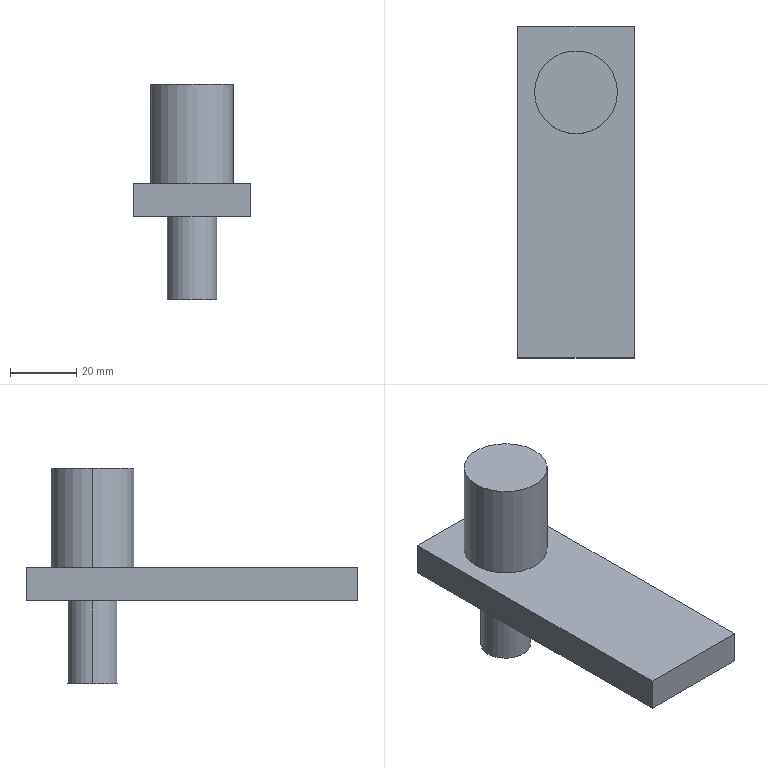Part | SolidWorks | features ICE 2, Extrusion 1 | 1 solid | 12 faces | box 35 x 100 x 65 mm | volume 54144 mm3 | plane 8 | cylinder 4 | commonest cylinder face diameters 15 x2 25 x2
STEP:
#1=CARTESIAN_POINT('',(-7.5,30.,-25.));
#2=VERTEX_POINT('',#1);
#3=CARTESIAN_POINT('',(7.5,30.,-25.));
#4=VERTEX_POINT('',#3);
#5=CARTESIAN_POINT('',(0.,30.,-25.));
#6=DIRECTION('',(0.,0.,-1.));
#7=DIRECTION('',(-1.,0.,0.));
#8=AXIS2_PLACEMENT_3D('',#5,#6,#7);
#9=CIRCLE('',#8,7.5);
#10=EDGE_CURVE('',#2,#4,#9,.T.);
#11=ORIENTED_EDGE('',*,*,#10,.F.);
#12=CARTESIAN_POINT('',(-7.5,30.,0.));
#13=VERTEX_POINT('',#12);
#14=CARTESIAN_POINT('',(-7.5,30.,-25.));
#15=DIRECTION('',(0.,0.,1.));
#16=VECTOR('',#15,1000.);
#17=LINE('',#14,#16);
#18=EDGE_CURVE('',#2,#13,#17,.T.);
#19=ORIENTED_EDGE('',*,*,#18,.T.);
#20=CARTESIAN_POINT('',(7.5,30.,0.));
#21=VERTEX_POINT('',#20);
#22=CARTESIAN_POINT('',(0.,30.,0.));
#23=DIRECTION('',(0.,0.,-1.));
#24=DIRECTION('',(-1.,0.,0.));
#25=AXIS2_PLACEMENT_3D('',#22,#23,#24);
#26=CIRCLE('',#25,7.5);
#27=EDGE_CURVE('',#13,#21,#26,.T.);
#28=ORIENTED_EDGE('',*,*,#27,.T.);
#29=CARTESIAN_POINT('',(7.5,30.,-25.));
#30=DIRECTION('',(0.,0.,1.));
#31=VECTOR('',#30,1000.);
#32=LINE('',#29,#31);
#33=EDGE_CURVE('',#4,#21,#32,.T.);
#34=ORIENTED_EDGE('',*,*,#33,.F.);
#35=EDGE_LOOP('',(#11,#19,#28,#34));
#36=FACE_OUTER_BOUND('',#35,.T.);
#37=CARTESIAN_POINT('',(0.,30.,-25.));
#38=DIRECTION('',(0.,0.,1.));
#39=DIRECTION('',(1.,0.,0.));
#40=AXIS2_PLACEMENT_3D('',#37,#38,#39);
#41=CYLINDRICAL_SURFACE('',#40,7.5);
#42=ADVANCED_FACE('',(#36),#41,.T.);
#43=CARTESIAN_POINT('',(12.5,30.,40.));
#44=VERTEX_POINT('',#43);
#45=CARTESIAN_POINT('',(-12.5,30.,40.));
#46=VERTEX_POINT('',#45);
#47=CARTESIAN_POINT('',(0.,30.,40.));
#48=DIRECTION('',(0.,0.,1.));
#49=DIRECTION('',(1.,0.,0.));
#50=AXIS2_PLACEMENT_3D('',#47,#48,#49);
#51=CIRCLE('',#50,12.5);
#52=EDGE_CURVE('',#44,#46,#51,.T.);
#53=ORIENTED_EDGE('',*,*,#52,.F.);
#54=CARTESIAN_POINT('',(12.5,30.,10.));
#55=VERTEX_POINT('',#54);
#56=CARTESIAN_POINT('',(12.5,30.,40.));
#57=DIRECTION('',(0.,0.,-1.));
#58=VECTOR('',#57,1000.);
#59=LINE('',#56,#58);
#60=EDGE_CURVE('',#44,#55,#59,.T.);
#61=ORIENTED_EDGE('',*,*,#60,.T.);
#62=CARTESIAN_POINT('',(-12.5,30.,10.));
#63=VERTEX_POINT('',#62);
#64=CARTESIAN_POINT('',(0.,30.,10.));
#65=DIRECTION('',(0.,0.,1.));
#66=DIRECTION('',(-1.,0.,0.));
#67=AXIS2_PLACEMENT_3D('',#64,#65,#66);
#68=CIRCLE('',#67,12.5);
#69=EDGE_CURVE('',#55,#63,#68,.T.);
#70=ORIENTED_EDGE('',*,*,#69,.T.);
#71=CARTESIAN_POINT('',(-12.5,30.,40.));
#72=DIRECTION('',(0.,0.,-1.));
#73=VECTOR('',#72,1000.);
#74=LINE('',#71,#73);
#75=EDGE_CURVE('',#46,#63,#74,.T.);
#76=ORIENTED_EDGE('',*,*,#75,.F.);
#77=EDGE_LOOP('',(#53,#61,#70,#76));
#78=FACE_OUTER_BOUND('',#77,.T.);
#79=CARTESIAN_POINT('',(0.,30.,40.));
#80=DIRECTION('',(0.,0.,-1.));
#81=DIRECTION('',(-1.,0.,0.));
#82=AXIS2_PLACEMENT_3D('',#79,#80,#81);
#83=CYLINDRICAL_SURFACE('',#82,12.5);
#84=ADVANCED_FACE('',(#78),#83,.T.);
#85=CARTESIAN_POINT('',(17.5,-50.,0.));
#86=VERTEX_POINT('',#85);
#87=CARTESIAN_POINT('',(17.5,50.,0.));
#88=VERTEX_POINT('',#87);
#89=CARTESIAN_POINT('',(17.5,-50.,0.));
#90=DIRECTION('',(0.,1.,0.));
#91=VECTOR('',#90,1000.);
#92=LINE('',#89,#91);
#93=EDGE_CURVE('',#86,#88,#92,.T.);
#94=ORIENTED_EDGE('',*,*,#93,.T.);
#95=CARTESIAN_POINT('',(17.5,50.,10.));
#96=VERTEX_POINT('',#95);
#97=CARTESIAN_POINT('',(17.5,50.,10.));
#98=DIRECTION('',(0.,0.,-1.));
#99=VECTOR('',#98,1000.);
#100=LINE('',#97,#99);
#101=EDGE_CURVE('',#96,#88,#100,.T.);
#102=ORIENTED_EDGE('',*,*,#101,.F.);
#103=CARTESIAN_POINT('',(17.5,-50.,10.));
#104=VERTEX_POINT('',#103);
#105=CARTESIAN_POINT('',(17.5,-50.,10.));
#106=DIRECTION('',(0.,1.,0.));
#107=VECTOR('',#106,1000.);
#108=LINE('',#105,#107);
#109=EDGE_CURVE('',#104,#96,#108,.T.);
#110=ORIENTED_EDGE('',*,*,#109,.F.);
#111=CARTESIAN_POINT('',(17.5,-50.,10.));
#112=DIRECTION('',(0.,0.,-1.));
#113=VECTOR('',#112,1000.);
#114=LINE('',#111,#113);
#115=EDGE_CURVE('',#104,#86,#114,.T.);
#116=ORIENTED_EDGE('',*,*,#115,.T.);
#117=EDGE_LOOP('',(#94,#102,#110,#116));
#118=FACE_OUTER_BOUND('',#117,.T.);
#119=CARTESIAN_POINT('',(17.5,-50.,10.));
#120=DIRECTION('',(-1.,0.,0.));
#121=DIRECTION('',(0.,0.,1.));
#122=AXIS2_PLACEMENT_3D('',#119,#120,#121);
#123=PLANE('',#122);
#124=ADVANCED_FACE('',(#118),#123,.F.);
#125=CARTESIAN_POINT('',(-17.5,50.,0.));
#126=VERTEX_POINT('',#125);
#127=CARTESIAN_POINT('',(-17.5,50.,0.));
#128=DIRECTION('',(-1.,0.,0.));
#129=VECTOR('',#128,1000.);
#130=LINE('',#127,#129);
#131=EDGE_CURVE('',#88,#126,#130,.T.);
#132=ORIENTED_EDGE('',*,*,#131,.T.);
#133=CARTESIAN_POINT('',(-17.5,50.,10.));
#134=VERTEX_POINT('',#133);
#135=CARTESIAN_POINT('',(-17.5,50.,10.));
#136=DIRECTION('',(0.,0.,-1.));
#137=VECTOR('',#136,1000.);
#138=LINE('',#135,#137);
#139=EDGE_CURVE('',#134,#126,#138,.T.);
#140=ORIENTED_EDGE('',*,*,#139,.F.);
#141=CARTESIAN_POINT('',(-17.5,50.,10.));
#142=DIRECTION('',(-1.,0.,0.));
#143=VECTOR('',#142,1000.);
#144=LINE('',#141,#143);
#145=EDGE_CURVE('',#96,#134,#144,.T.);
#146=ORIENTED_EDGE('',*,*,#145,.F.);
#147=ORIENTED_EDGE('',*,*,#101,.T.);
#148=EDGE_LOOP('',(#132,#140,#146,#147));
#149=FACE_OUTER_BOUND('',#148,.T.);
#150=CARTESIAN_POINT('',(-17.5,50.,10.));
#151=DIRECTION('',(0.,-1.,0.));
#152=DIRECTION('',(0.,0.,-1.));
#153=AXIS2_PLACEMENT_3D('',#150,#151,#152);
#154=PLANE('',#153);
#155=ADVANCED_FACE('',(#149),#154,.F.);
#156=CARTESIAN_POINT('',(-17.5,-50.,0.));
#157=VERTEX_POINT('',#156);
#158=CARTESIAN_POINT('',(-17.5,-50.,0.));
#159=DIRECTION('',(0.,-1.,0.));
#160=VECTOR('',#159,1000.);
#161=LINE('',#158,#160);
#162=EDGE_CURVE('',#126,#157,#161,.T.);
#163=ORIENTED_EDGE('',*,*,#162,.T.);
#164=CARTESIAN_POINT('',(-17.5,-50.,10.));
#165=VERTEX_POINT('',#164);
#166=CARTESIAN_POINT('',(-17.5,-50.,10.));
#167=DIRECTION('',(0.,0.,-1.));
#168=VECTOR('',#167,1000.);
#169=LINE('',#166,#168);
#170=EDGE_CURVE('',#165,#157,#169,.T.);
#171=ORIENTED_EDGE('',*,*,#170,.F.);
#172=CARTESIAN_POINT('',(-17.5,-50.,10.));
#173=DIRECTION('',(0.,-1.,0.));
#174=VECTOR('',#173,1000.);
#175=LINE('',#172,#174);
#176=EDGE_CURVE('',#134,#165,#175,.T.);
#177=ORIENTED_EDGE('',*,*,#176,.F.);
#178=ORIENTED_EDGE('',*,*,#139,.T.);
#179=EDGE_LOOP('',(#163,#171,#177,#178));
#180=FACE_OUTER_BOUND('',#179,.T.);
#181=CARTESIAN_POINT('',(-17.5,-50.,10.));
#182=DIRECTION('',(1.,0.,0.));
#183=DIRECTION('',(0.,0.,-1.));
#184=AXIS2_PLACEMENT_3D('',#181,#182,#183);
#185=PLANE('',#184);
#186=ADVANCED_FACE('',(#180),#185,.F.);
#187=CARTESIAN_POINT('',(-17.5,-50.,0.));
#188=DIRECTION('',(1.,0.,0.));
#189=VECTOR('',#188,1000.);
#190=LINE('',#187,#189);
#191=EDGE_CURVE('',#157,#86,#190,.T.);
#192=ORIENTED_EDGE('',*,*,#191,.T.);
#193=ORIENTED_EDGE('',*,*,#115,.F.);
#194=CARTESIAN_POINT('',(-17.5,-50.,10.));
#195=DIRECTION('',(1.,0.,0.));
#196=VECTOR('',#195,1000.);
#197=LINE('',#194,#196);
#198=EDGE_CURVE('',#165,#104,#197,.T.);
#199=ORIENTED_EDGE('',*,*,#198,.F.);
#200=ORIENTED_EDGE('',*,*,#170,.T.);
#201=EDGE_LOOP('',(#192,#193,#199,#200));
#202=FACE_OUTER_BOUND('',#201,.T.);
#203=CARTESIAN_POINT('',(-17.5,-50.,10.));
#204=DIRECTION('',(0.,1.,0.));
#205=DIRECTION('',(0.,0.,1.));
#206=AXIS2_PLACEMENT_3D('',#203,#204,#205);
#207=PLANE('',#206);
#208=ADVANCED_FACE('',(#202),#207,.F.);
#209=CARTESIAN_POINT('',(0.,30.,10.));
#210=DIRECTION('',(0.,0.,1.));
#211=DIRECTION('',(-1.,0.,0.));
#212=AXIS2_PLACEMENT_3D('',#209,#210,#211);
#213=CIRCLE('',#212,12.5);
#214=EDGE_CURVE('',#63,#55,#213,.T.);
#215=ORIENTED_EDGE('',*,*,#214,.F.);
#216=ORIENTED_EDGE('',*,*,#69,.F.);
#217=EDGE_LOOP('',(#215,#216));
#218=FACE_BOUND('',#217,.T.);
#219=ORIENTED_EDGE('',*,*,#109,.T.);
#220=ORIENTED_EDGE('',*,*,#145,.T.);
#221=ORIENTED_EDGE('',*,*,#176,.T.);
#222=ORIENTED_EDGE('',*,*,#198,.T.);
#223=EDGE_LOOP('',(#219,#220,#221,#222));
#224=FACE_OUTER_BOUND('',#223,.T.);
#225=CARTESIAN_POINT('',(0.,0.,10.));
#226=DIRECTION('',(0.,0.,-1.));
#227=DIRECTION('',(-1.,0.,0.));
#228=AXIS2_PLACEMENT_3D('',#225,#226,#227);
#229=PLANE('',#228);
#230=ADVANCED_FACE('',(#218,#224),#229,.F.);
#231=CARTESIAN_POINT('',(0.,30.,0.));
#232=DIRECTION('',(0.,0.,-1.));
#233=DIRECTION('',(-1.,0.,0.));
#234=AXIS2_PLACEMENT_3D('',#231,#232,#233);
#235=CIRCLE('',#234,7.5);
#236=EDGE_CURVE('',#21,#13,#235,.T.);
#237=ORIENTED_EDGE('',*,*,#236,.F.);
#238=ORIENTED_EDGE('',*,*,#27,.F.);
#239=EDGE_LOOP('',(#237,#238));
#240=FACE_BOUND('',#239,.T.);
#241=ORIENTED_EDGE('',*,*,#93,.F.);
#242=ORIENTED_EDGE('',*,*,#191,.F.);
#243=ORIENTED_EDGE('',*,*,#162,.F.);
#244=ORIENTED_EDGE('',*,*,#131,.F.);
#245=EDGE_LOOP('',(#241,#242,#243,#244));
#246=FACE_OUTER_BOUND('',#245,.T.);
#247=CARTESIAN_POINT('',(0.,0.,0.));
#248=DIRECTION('',(0.,0.,-1.));
#249=DIRECTION('',(-1.,0.,0.));
#250=AXIS2_PLACEMENT_3D('',#247,#248,#249);
#251=PLANE('',#250);
#252=ADVANCED_FACE('',(#240,#246),#251,.T.);
#253=ORIENTED_EDGE('',*,*,#60,.F.);
#254=CARTESIAN_POINT('',(0.,30.,40.));
#255=DIRECTION('',(0.,0.,1.));
#256=DIRECTION('',(1.,0.,0.));
#257=AXIS2_PLACEMENT_3D('',#254,#255,#256);
#258=CIRCLE('',#257,12.5);
#259=EDGE_CURVE('',#46,#44,#258,.T.);
#260=ORIENTED_EDGE('',*,*,#259,.F.);
#261=ORIENTED_EDGE('',*,*,#75,.T.);
#262=ORIENTED_EDGE('',*,*,#214,.T.);
#263=EDGE_LOOP('',(#253,#260,#261,#262));
#264=FACE_OUTER_BOUND('',#263,.T.);
#265=CARTESIAN_POINT('',(0.,30.,40.));
#266=DIRECTION('',(0.,0.,-1.));
#267=DIRECTION('',(-1.,0.,0.));
#268=AXIS2_PLACEMENT_3D('',#265,#266,#267);
#269=CYLINDRICAL_SURFACE('',#268,12.5);
#270=ADVANCED_FACE('',(#264),#269,.T.);
#271=ORIENTED_EDGE('',*,*,#259,.T.);
#272=ORIENTED_EDGE('',*,*,#52,.T.);
#273=EDGE_LOOP('',(#271,#272));
#274=FACE_OUTER_BOUND('',#273,.T.);
#275=CARTESIAN_POINT('',(0.,30.,40.));
#276=DIRECTION('',(0.,0.,1.));
#277=DIRECTION('',(1.,0.,0.));
#278=AXIS2_PLACEMENT_3D('',#275,#276,#277);
#279=PLANE('',#278);
#280=ADVANCED_FACE('',(#274),#279,.T.);
#281=ORIENTED_EDGE('',*,*,#18,.F.);
#282=CARTESIAN_POINT('',(0.,30.,-25.));
#283=DIRECTION('',(0.,0.,-1.));
#284=DIRECTION('',(-1.,0.,0.));
#285=AXIS2_PLACEMENT_3D('',#282,#283,#284);
#286=CIRCLE('',#285,7.5);
#287=EDGE_CURVE('',#4,#2,#286,.T.);
#288=ORIENTED_EDGE('',*,*,#287,.F.);
#289=ORIENTED_EDGE('',*,*,#33,.T.);
#290=ORIENTED_EDGE('',*,*,#236,.T.);
#291=EDGE_LOOP('',(#281,#288,#289,#290));
#292=FACE_OUTER_BOUND('',#291,.T.);
#293=CARTESIAN_POINT('',(0.,30.,-25.));
#294=DIRECTION('',(0.,0.,1.));
#295=DIRECTION('',(1.,0.,0.));
#296=AXIS2_PLACEMENT_3D('',#293,#294,#295);
#297=CYLINDRICAL_SURFACE('',#296,7.5);
#298=ADVANCED_FACE('',(#292),#297,.T.);
#299=ORIENTED_EDGE('',*,*,#287,.T.);
#300=ORIENTED_EDGE('',*,*,#10,.T.);
#301=EDGE_LOOP('',(#299,#300));
#302=FACE_OUTER_BOUND('',#301,.T.);
#303=CARTESIAN_POINT('',(0.,30.,-25.));
#304=DIRECTION('',(0.,0.,-1.));
#305=DIRECTION('',(-1.,0.,0.));
#306=AXIS2_PLACEMENT_3D('',#303,#304,#305);
#307=PLANE('',#306);
#308=ADVANCED_FACE('',(#302),#307,.T.);
#309=CLOSED_SHELL('',(#42,#84,#124,#155,#186,#208,#230,#252,#270,#280,#298,#308));
#310=MANIFOLD_SOLID_BREP('',#309);
#311=CARTESIAN_POINT('',(0.,0.,0.));
#312=DIRECTION('',(0.,0.,1.));
#313=DIRECTION('',(1.,0.,0.));
#314=AXIS2_PLACEMENT_3D('',#311,#312,#313);
#315=(LENGTH_UNIT()NAMED_UNIT(*)SI_UNIT(.MILLI.,.METRE.));
#316=UNCERTAINTY_MEASURE_WITH_UNIT(LENGTH_MEASURE(0.00001),#315,'','');
#317=(NAMED_UNIT(*)PLANE_ANGLE_UNIT()SI_UNIT($,.RADIAN.));
#318=(NAMED_UNIT(*)SI_UNIT($,.STERADIAN.)SOLID_ANGLE_UNIT());
#319=(GEOMETRIC_REPRESENTATION_CONTEXT(3)GLOBAL_UNCERTAINTY_ASSIGNED_CONTEXT((#316))GLOBAL_UNIT_ASSIGNED_CONTEXT((#315,#317,#318))REPRESENTATION_CONTEXT('',''));
#320=ADVANCED_BREP_SHAPE_REPRESENTATION('',(#310,#314),#319);